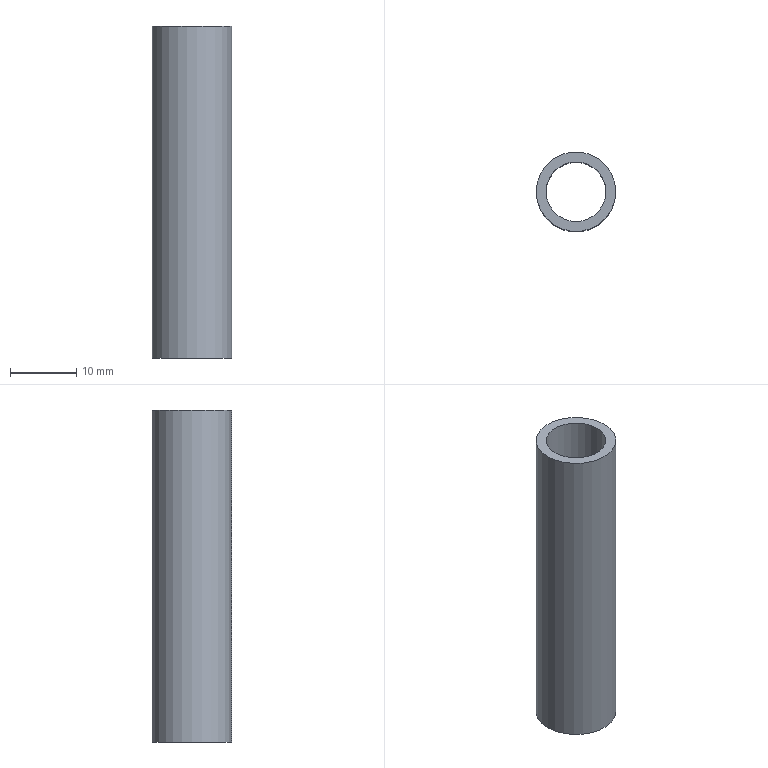Part | STEP file | BS EN 10305-4 - E235 - 12 x 1,5 - 50 | 1 solid | 4 faces | box 12 x 12 x 50 mm | volume 2474 mm3 | cylinder 2 | plane 2 | commonest cylinder face diameters 9 x1 12 x1
STEP:
#1=CARTESIAN_POINT('',(0.,0.,0.));
#2=DIRECTION('',(0.,0.,1.));
#3=DIRECTION('',(1.,0.,0.));
#4=AXIS2_PLACEMENT_3D('',#1,#2,#3);
#5=CARTESIAN_POINT('',(4.5,0.,50.));
#6=VERTEX_POINT('',#5);
#7=CARTESIAN_POINT('',(0.,0.,50.));
#8=DIRECTION('',(0.,0.,1.));
#9=DIRECTION('',(-1.,0.,0.));
#10=AXIS2_PLACEMENT_3D('',#7,#8,#9);
#11=CIRCLE('',#10,4.5);
#12=CARTESIAN_POINT('',(0.,0.,0.));
#13=DIRECTION('',(0.,0.,1.));
#14=DIRECTION('',(-1.,0.,0.));
#15=AXIS2_PLACEMENT_3D('',#12,#13,#14);
#16=CYLINDRICAL_SURFACE('',#15,4.5);
#17=CARTESIAN_POINT('',(0.,50.));
#18=DIRECTION('',(1.,0.));
#19=VECTOR('',#18,1.);
#20=LINE('',#17,#19);
#21=(GEOMETRIC_REPRESENTATION_CONTEXT(2)PARAMETRIC_REPRESENTATION_CONTEXT()REPRESENTATION_CONTEXT('',''));
#22=DEFINITIONAL_REPRESENTATION('',(#20),#21);
#23=PCURVE('',#16,#22);
#24=CARTESIAN_POINT('',(0.,0.,50.));
#25=DIRECTION('',(0.,0.,1.));
#26=DIRECTION('',(1.,0.,0.));
#27=AXIS2_PLACEMENT_3D('',#24,#25,#26);
#28=PLANE('',#27);
#29=CARTESIAN_POINT('',(0.,0.));
#30=DIRECTION('',(-1.,0.));
#31=AXIS2_PLACEMENT_2D('',#29,#30);
#32=CIRCLE('',#31,4.5);
#33=(GEOMETRIC_REPRESENTATION_CONTEXT(2)PARAMETRIC_REPRESENTATION_CONTEXT()REPRESENTATION_CONTEXT('',''));
#34=DEFINITIONAL_REPRESENTATION('',(#32),#33);
#35=PCURVE('',#28,#34);
#36=SURFACE_CURVE('',#11,(#23,#35),.PCURVE_S1.);
#37=EDGE_CURVE('',#6,#6,#36,.T.);
#38=ORIENTED_EDGE('',*,*,#37,.F.);
#39=CARTESIAN_POINT('',(4.5,0.,0.));
#40=VERTEX_POINT('',#39);
#41=CARTESIAN_POINT('',(4.5,0.,0.));
#42=CARTESIAN_POINT('',(4.5,0.,50.));
#43=B_SPLINE_CURVE_WITH_KNOTS('',1,(#41,#42),.UNSPECIFIED.,.F.,.F.,(2,2),(0.,50.),.PIECEWISE_BEZIER_KNOTS.);
#44=CARTESIAN_POINT('',(3.142,0.));
#45=DIRECTION('',(0.,1.));
#46=VECTOR('',#45,1.);
#47=LINE('',#44,#46);
#48=(GEOMETRIC_REPRESENTATION_CONTEXT(2)PARAMETRIC_REPRESENTATION_CONTEXT()REPRESENTATION_CONTEXT('',''));
#49=DEFINITIONAL_REPRESENTATION('',(#47),#48);
#50=PCURVE('',#16,#49);
#51=CARTESIAN_POINT('',(9.425,0.));
#52=DIRECTION('',(0.,1.));
#53=VECTOR('',#52,1.);
#54=LINE('',#51,#53);
#55=(GEOMETRIC_REPRESENTATION_CONTEXT(2)PARAMETRIC_REPRESENTATION_CONTEXT()REPRESENTATION_CONTEXT('',''));
#56=DEFINITIONAL_REPRESENTATION('',(#54),#55);
#57=PCURVE('',#16,#56);
#58=SEAM_CURVE('',#43,(#50,#57),.PCURVE_S1.);
#59=EDGE_CURVE('',#40,#6,#58,.T.);
#60=ORIENTED_EDGE('',*,*,#59,.F.);
#61=CARTESIAN_POINT('',(0.,0.,0.));
#62=DIRECTION('',(0.,0.,1.));
#63=DIRECTION('',(-1.,0.,0.));
#64=AXIS2_PLACEMENT_3D('',#61,#62,#63);
#65=CIRCLE('',#64,4.5);
#66=CARTESIAN_POINT('',(0.,0.));
#67=DIRECTION('',(1.,0.));
#68=VECTOR('',#67,1.);
#69=LINE('',#66,#68);
#70=(GEOMETRIC_REPRESENTATION_CONTEXT(2)PARAMETRIC_REPRESENTATION_CONTEXT()REPRESENTATION_CONTEXT('',''));
#71=DEFINITIONAL_REPRESENTATION('',(#69),#70);
#72=PCURVE('',#16,#71);
#73=CARTESIAN_POINT('',(0.,0.,0.));
#74=DIRECTION('',(0.,0.,1.));
#75=DIRECTION('',(1.,0.,0.));
#76=AXIS2_PLACEMENT_3D('',#73,#74,#75);
#77=PLANE('',#76);
#78=CARTESIAN_POINT('',(0.,0.));
#79=DIRECTION('',(-1.,0.));
#80=AXIS2_PLACEMENT_2D('',#78,#79);
#81=CIRCLE('',#80,4.5);
#82=(GEOMETRIC_REPRESENTATION_CONTEXT(2)PARAMETRIC_REPRESENTATION_CONTEXT()REPRESENTATION_CONTEXT('',''));
#83=DEFINITIONAL_REPRESENTATION('',(#81),#82);
#84=PCURVE('',#77,#83);
#85=SURFACE_CURVE('',#65,(#72,#84),.PCURVE_S1.);
#86=EDGE_CURVE('',#40,#40,#85,.T.);
#87=ORIENTED_EDGE('',*,*,#86,.T.);
#88=ORIENTED_EDGE('',*,*,#59,.T.);
#89=EDGE_LOOP('',(#38,#60,#87,#88));
#90=FACE_BOUND('',#89,.F.);
#91=ADVANCED_FACE('',(#90),#16,.F.);
#92=CARTESIAN_POINT('',(6.,0.,50.));
#93=VERTEX_POINT('',#92);
#94=CARTESIAN_POINT('',(0.,0.,50.));
#95=DIRECTION('',(0.,0.,-1.));
#96=DIRECTION('',(-1.,0.,0.));
#97=AXIS2_PLACEMENT_3D('',#94,#95,#96);
#98=CIRCLE('',#97,6.);
#99=CARTESIAN_POINT('',(0.,0.,0.));
#100=DIRECTION('',(0.,0.,1.));
#101=DIRECTION('',(-1.,0.,0.));
#102=AXIS2_PLACEMENT_3D('',#99,#100,#101);
#103=CYLINDRICAL_SURFACE('',#102,6.);
#104=CARTESIAN_POINT('',(12.566,50.));
#105=DIRECTION('',(-1.,0.));
#106=VECTOR('',#105,1.);
#107=LINE('',#104,#106);
#108=(GEOMETRIC_REPRESENTATION_CONTEXT(2)PARAMETRIC_REPRESENTATION_CONTEXT()REPRESENTATION_CONTEXT('',''));
#109=DEFINITIONAL_REPRESENTATION('',(#107),#108);
#110=PCURVE('',#103,#109);
#111=CARTESIAN_POINT('',(-6.,0.));
#112=CARTESIAN_POINT('',(-6.,10.392));
#113=CARTESIAN_POINT('',(3.,5.196));
#114=CARTESIAN_POINT('',(12.,0.));
#115=CARTESIAN_POINT('',(3.,-5.196));
#116=CARTESIAN_POINT('',(-6.,-10.392));
#117=CARTESIAN_POINT('',(-6.,0.));
#118=(BOUNDED_CURVE()B_SPLINE_CURVE(2,(#111,#112,#113,#114,#115,#116,#117),.UNSPECIFIED.,.T.,.F.)B_SPLINE_CURVE_WITH_KNOTS((1,2,2,2,2,1),(-2.094,0.,2.094,4.189,6.283,8.378),.UNSPECIFIED.)CURVE()GEOMETRIC_REPRESENTATION_ITEM()RATIONAL_B_SPLINE_CURVE((1.,0.5,1.,0.5,1.,0.5,1.))REPRESENTATION_ITEM(''));
#119=(GEOMETRIC_REPRESENTATION_CONTEXT(2)PARAMETRIC_REPRESENTATION_CONTEXT()REPRESENTATION_CONTEXT('',''));
#120=DEFINITIONAL_REPRESENTATION('',(#118),#119);
#121=PCURVE('',#28,#120);
#122=SURFACE_CURVE('',#98,(#110,#121),.PCURVE_S1.);
#123=EDGE_CURVE('',#93,#93,#122,.T.);
#124=ORIENTED_EDGE('',*,*,#123,.T.);
#125=CARTESIAN_POINT('',(6.,0.,0.));
#126=VERTEX_POINT('',#125);
#127=CARTESIAN_POINT('',(6.,0.,0.));
#128=CARTESIAN_POINT('',(6.,0.,50.));
#129=B_SPLINE_CURVE_WITH_KNOTS('',1,(#127,#128),.UNSPECIFIED.,.F.,.F.,(2,2),(0.,50.),.PIECEWISE_BEZIER_KNOTS.);
#130=CARTESIAN_POINT('',(3.142,0.));
#131=DIRECTION('',(0.,1.));
#132=VECTOR('',#131,1.);
#133=LINE('',#130,#132);
#134=(GEOMETRIC_REPRESENTATION_CONTEXT(2)PARAMETRIC_REPRESENTATION_CONTEXT()REPRESENTATION_CONTEXT('',''));
#135=DEFINITIONAL_REPRESENTATION('',(#133),#134);
#136=PCURVE('',#103,#135);
#137=CARTESIAN_POINT('',(9.425,0.));
#138=DIRECTION('',(0.,1.));
#139=VECTOR('',#138,1.);
#140=LINE('',#137,#139);
#141=(GEOMETRIC_REPRESENTATION_CONTEXT(2)PARAMETRIC_REPRESENTATION_CONTEXT()REPRESENTATION_CONTEXT('',''));
#142=DEFINITIONAL_REPRESENTATION('',(#140),#141);
#143=PCURVE('',#103,#142);
#144=SEAM_CURVE('',#129,(#136,#143),.PCURVE_S1.);
#145=EDGE_CURVE('',#126,#93,#144,.T.);
#146=ORIENTED_EDGE('',*,*,#145,.F.);
#147=CARTESIAN_POINT('',(0.,0.,0.));
#148=DIRECTION('',(0.,0.,-1.));
#149=DIRECTION('',(-1.,0.,0.));
#150=AXIS2_PLACEMENT_3D('',#147,#148,#149);
#151=CIRCLE('',#150,6.);
#152=CARTESIAN_POINT('',(12.566,0.));
#153=DIRECTION('',(-1.,0.));
#154=VECTOR('',#153,1.);
#155=LINE('',#152,#154);
#156=(GEOMETRIC_REPRESENTATION_CONTEXT(2)PARAMETRIC_REPRESENTATION_CONTEXT()REPRESENTATION_CONTEXT('',''));
#157=DEFINITIONAL_REPRESENTATION('',(#155),#156);
#158=PCURVE('',#103,#157);
#159=CARTESIAN_POINT('',(-6.,0.));
#160=CARTESIAN_POINT('',(-6.,10.392));
#161=CARTESIAN_POINT('',(3.,5.196));
#162=CARTESIAN_POINT('',(12.,0.));
#163=CARTESIAN_POINT('',(3.,-5.196));
#164=CARTESIAN_POINT('',(-6.,-10.392));
#165=CARTESIAN_POINT('',(-6.,0.));
#166=(BOUNDED_CURVE()B_SPLINE_CURVE(2,(#159,#160,#161,#162,#163,#164,#165),.UNSPECIFIED.,.T.,.F.)B_SPLINE_CURVE_WITH_KNOTS((1,2,2,2,2,1),(-2.094,0.,2.094,4.189,6.283,8.378),.UNSPECIFIED.)CURVE()GEOMETRIC_REPRESENTATION_ITEM()RATIONAL_B_SPLINE_CURVE((1.,0.5,1.,0.5,1.,0.5,1.))REPRESENTATION_ITEM(''));
#167=(GEOMETRIC_REPRESENTATION_CONTEXT(2)PARAMETRIC_REPRESENTATION_CONTEXT()REPRESENTATION_CONTEXT('',''));
#168=DEFINITIONAL_REPRESENTATION('',(#166),#167);
#169=PCURVE('',#77,#168);
#170=SURFACE_CURVE('',#151,(#158,#169),.PCURVE_S1.);
#171=EDGE_CURVE('',#126,#126,#170,.T.);
#172=ORIENTED_EDGE('',*,*,#171,.F.);
#173=ORIENTED_EDGE('',*,*,#145,.T.);
#174=EDGE_LOOP('',(#124,#146,#172,#173));
#175=FACE_BOUND('',#174,.T.);
#176=ADVANCED_FACE('',(#175),#103,.T.);
#177=ORIENTED_EDGE('',*,*,#171,.T.);
#178=EDGE_LOOP('',(#177));
#179=FACE_BOUND('',#178,.T.);
#180=ORIENTED_EDGE('',*,*,#86,.T.);
#181=EDGE_LOOP('',(#180));
#182=FACE_BOUND('',#181,.T.);
#183=ADVANCED_FACE('',(#179,#182),#77,.F.);
#184=ORIENTED_EDGE('',*,*,#123,.F.);
#185=EDGE_LOOP('',(#184));
#186=FACE_BOUND('',#185,.T.);
#187=ORIENTED_EDGE('',*,*,#37,.F.);
#188=EDGE_LOOP('',(#187));
#189=FACE_BOUND('',#188,.T.);
#190=ADVANCED_FACE('',(#186,#189),#28,.T.);
#191=CLOSED_SHELL('',(#91,#176,#183,#190));
#192=MANIFOLD_SOLID_BREP('',#191);
#193=(LENGTH_UNIT()NAMED_UNIT(*)SI_UNIT(.MILLI.,.METRE.));
#194=UNCERTAINTY_MEASURE_WITH_UNIT(LENGTH_MEASURE(0.00001),#193,'','');
#195=(NAMED_UNIT(*)PLANE_ANGLE_UNIT()SI_UNIT($,.RADIAN.));
#196=(NAMED_UNIT(*)SI_UNIT($,.STERADIAN.)SOLID_ANGLE_UNIT());
#197=(GEOMETRIC_REPRESENTATION_CONTEXT(3)GLOBAL_UNCERTAINTY_ASSIGNED_CONTEXT((#194))GLOBAL_UNIT_ASSIGNED_CONTEXT((#193,#195,#196))REPRESENTATION_CONTEXT('',''));
#198=ADVANCED_BREP_SHAPE_REPRESENTATION('',(#4,#192),#197);